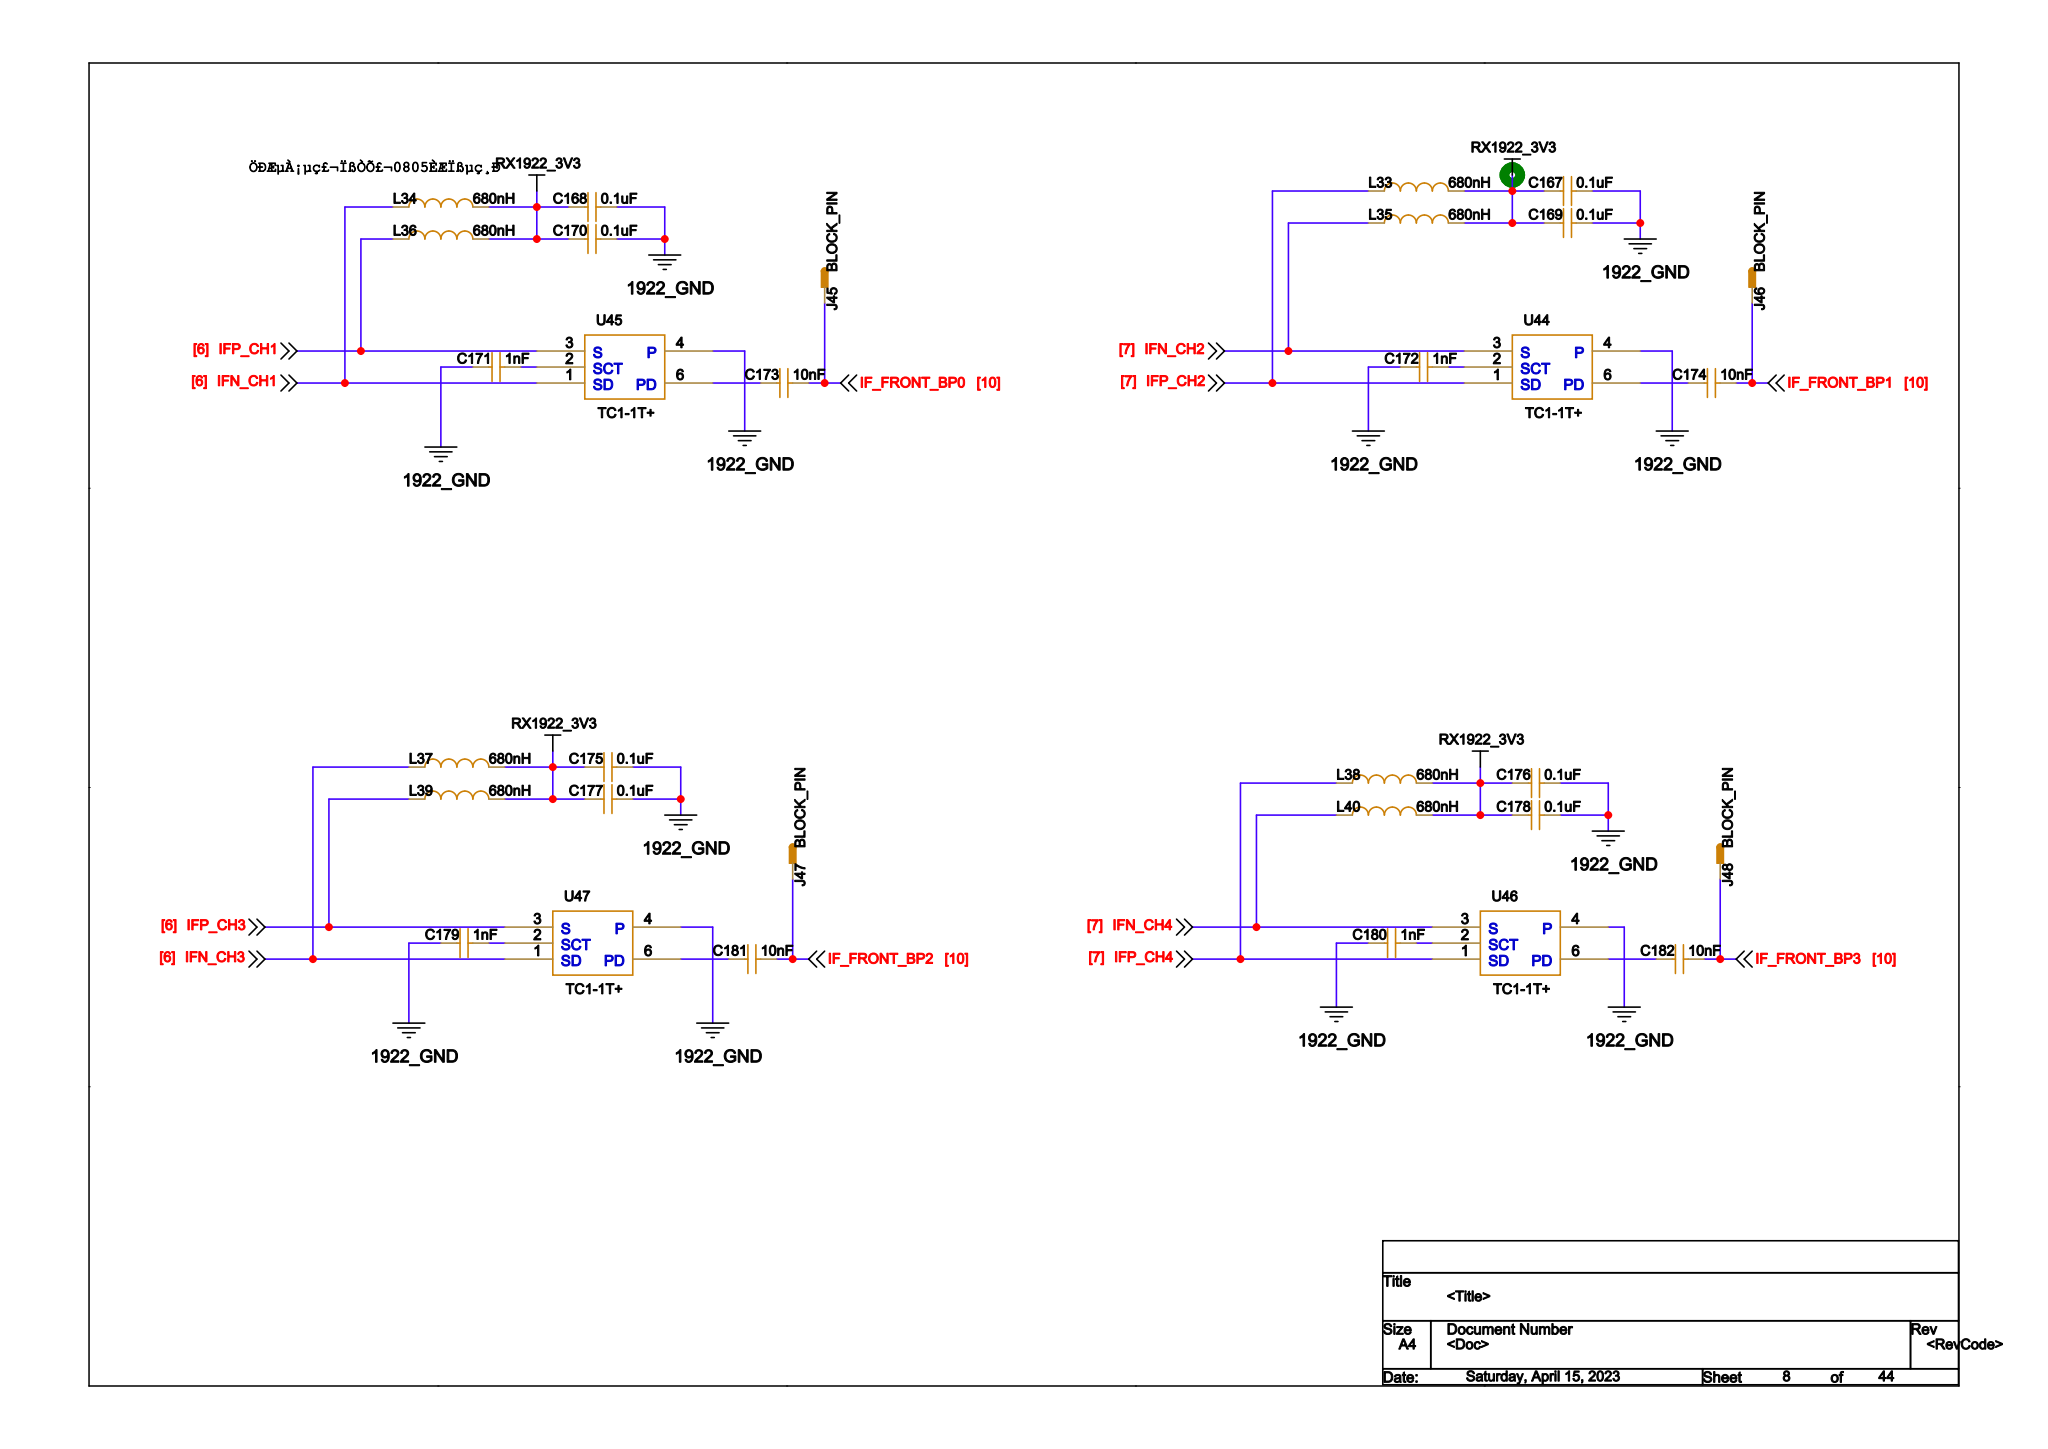Circuit board | Cadence Allegro | 1034 parts | 912 nets | one sheet of the schematic
Parts on this sheet (reference | value | footprint):
C167 | 0.1uF | C0402
C168 | 0.1uF | C0402
C169 | 0.1uF | C0402
C170 | 0.1uF | C0402
C171 | 1nF | C0402
C172 | 1nF | C0402
C173 | 10nF | C0402
C174 | 10nF | C0402
C175 | 0.1uF | C0402
C176 | 0.1uF | C0402
C177 | 0.1uF | C0402
C178 | 0.1uF | C0402
C179 | 1nF | C0402
C180 | 1nF | C0402
C181 | 10nF | C0402
C182 | 10nF | C0402
J45 | BLOCK_PIN | B_PIN_SMD
J46 | BLOCK_PIN | B_PIN_SMD
J47 | BLOCK_PIN | B_PIN_SMD
J48 | BLOCK_PIN | B_PIN_SMD
L33 | 680nH | L0805
L34 | 680nH | L0805
L35 | 680nH | L0805
L36 | 680nH | L0805
L37 | 680nH | L0805
L38 | 680nH | L0805
L39 | 680nH | L0805
L40 | 680nH | L0805
U44 | TC1-1T+ | TC1_1T_SMD
U45 | TC1-1T+ | TC1_1T_SMD
U46 | TC1-1T+ | TC1_1T_SMD
U47 | TC1-1T+ | TC1_1T_SMD
Nets of these parts (net: part-pin ...):
IF_FRONT_BP0_D1: C173-2 J45-1
IF_FRONT_BP1_D1: C174-2 J46-1
IF_FRONT_BP2_D1: C181-2 J47-1
IF_FRONT_BP3_D1: C182-2 J48-1
1922_GND: C167-2 C168-2 C169-2 C170-2 C171-1 C172-1 C175-2 C176-2 C177-2 C178-2 C179-1 C180-1 U44-4 U45-4 U46-4 U47-4
PWR1922_3V3_1: C167-1 C168-1 C169-1 C170-1 C175-1 C176-1 C177-1 C178-1 L33-2 L34-2 L35-2 L36-2 L37-2 L38-2 L39-2 L40-2
N156926_D1: C173-1 U45-6
N157763_D1: C174-1 U44-6
N158323_D1: C181-1 U47-6
N158912_D1: C182-1 U46-6
N156737_D1: C171-2 U45-2
N157727_D1: C172-2 U44-2
N158287_D1: C179-2 U47-2
N158876_D1: C180-2 U46-2
IFP_CH2_D1: L33-1 U44-1
IFN_CH1_D1: L34-1 U45-1
IFN_CH2_D1: L35-1 U44-3
IFP_CH1_D1: L36-1 U45-3
IFN_CH3_D1: L37-1 U47-1
IFP_CH4_D1: L38-1 U46-1
IFP_CH3_D1: L39-1 U47-3
IFN_CH4_D1: L40-1 U46-3